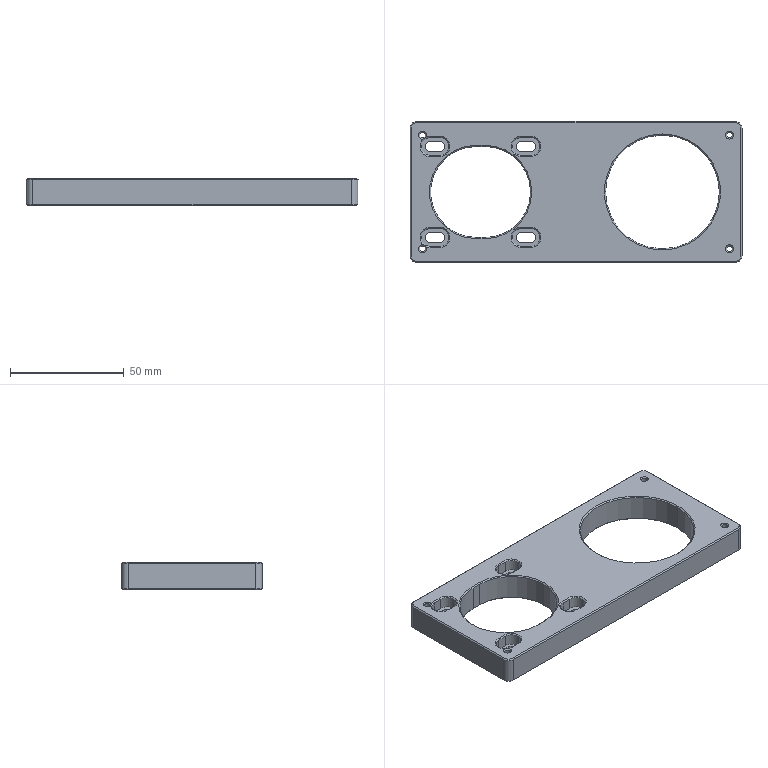Part | SolidWorks | features BaseBody 1 | 1 solid | 151 faces | box 146 x 62 x 12 mm | volume 64829 mm3 | plane 56 | cone 54 | cylinder 41 | commonest cylinder face diameters 4.5 x12 8 x12 2.5 x8 6 x4 40 x3 50 x2